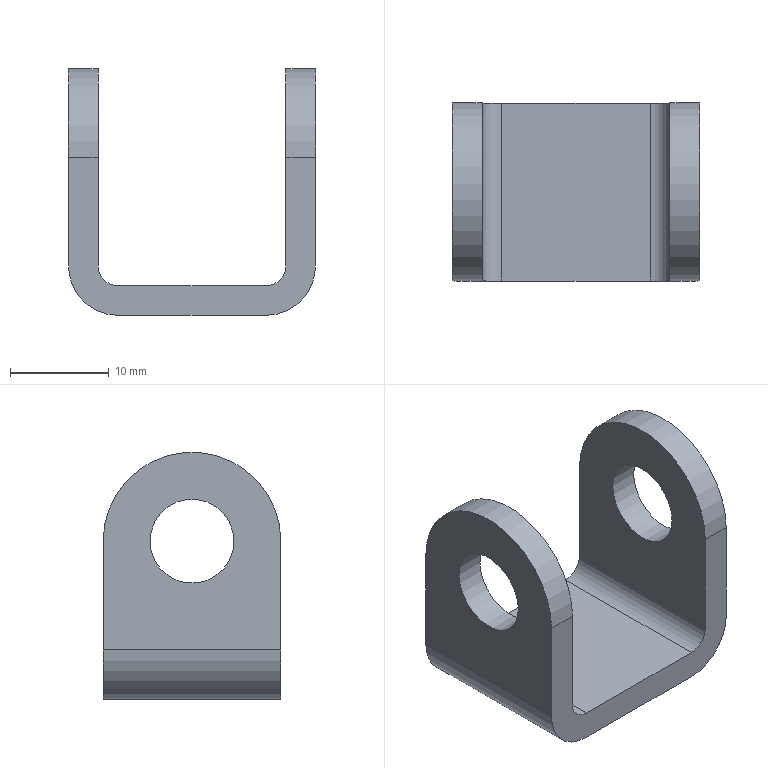Part | NX | features DATUM_CSYS 6, EXTRUDE 5, SKETCH 5, EXTRACT_FACE 4, BLEND 2, Instance Feature 1, Mirror Feature 1 | 1 solid | 16 faces | box 25 x 18 x 25 mm | volume 3015 mm3 | plane 8 | cylinder 8 | commonest cylinder face diameters 4 x2 8.5 x2 10 x2 18 x2
STEP:
#1=CARTESIAN_POINT('',(-12.5,9.,16.));
#2=VERTEX_POINT('',#1);
#3=CARTESIAN_POINT('',(-12.5,9.,5.));
#4=VERTEX_POINT('',#3);
#5=CARTESIAN_POINT('',(-12.5,9.,3.));
#6=DIRECTION('',(0.,0.,-1.));
#7=VECTOR('',#6,1000.);
#8=LINE('',#5,#7);
#9=EDGE_CURVE('',#2,#4,#8,.T.);
#10=ORIENTED_EDGE('',*,*,#9,.T.);
#11=CARTESIAN_POINT('',(-12.5,-9.,5.));
#12=VERTEX_POINT('',#11);
#13=CARTESIAN_POINT('',(-12.5,9.,5.));
#14=DIRECTION('',(0.,-1.,0.));
#15=VECTOR('',#14,1000.);
#16=LINE('',#13,#15);
#17=EDGE_CURVE('',#4,#12,#16,.T.);
#18=ORIENTED_EDGE('',*,*,#17,.T.);
#19=CARTESIAN_POINT('',(-12.5,-9.,16.));
#20=VERTEX_POINT('',#19);
#21=CARTESIAN_POINT('',(-12.5,-9.,3.));
#22=DIRECTION('',(0.,0.,-1.));
#23=VECTOR('',#22,1000.);
#24=LINE('',#21,#23);
#25=EDGE_CURVE('',#20,#12,#24,.T.);
#26=ORIENTED_EDGE('',*,*,#25,.F.);
#27=CARTESIAN_POINT('',(-12.5,0.,16.));
#28=DIRECTION('',(-1.,0.,0.));
#29=DIRECTION('',(0.,-1.,0.));
#30=AXIS2_PLACEMENT_3D('',#27,#28,#29);
#31=CIRCLE('',#30,9.);
#32=EDGE_CURVE('',#20,#2,#31,.T.);
#33=ORIENTED_EDGE('',*,*,#32,.T.);
#34=EDGE_LOOP('',(#10,#18,#26,#33));
#35=FACE_BOUND('',#34,.T.);
#36=CARTESIAN_POINT('',(-12.5,-4.25,16.));
#37=VERTEX_POINT('',#36);
#38=CARTESIAN_POINT('',(-12.5,0.,16.));
#39=DIRECTION('',(-1.,0.,0.));
#40=DIRECTION('',(0.,-1.,0.));
#41=AXIS2_PLACEMENT_3D('',#38,#39,#40);
#42=CIRCLE('',#41,4.25);
#43=EDGE_CURVE('',#37,#37,#42,.T.);
#44=ORIENTED_EDGE('',*,*,#43,.F.);
#45=EDGE_LOOP('',(#44));
#46=FACE_BOUND('',#45,.T.);
#47=CARTESIAN_POINT('',(-12.5,9.,3.));
#48=DIRECTION('',(1.,0.,0.));
#49=DIRECTION('',(0.,1.,0.));
#50=AXIS2_PLACEMENT_3D('',#47,#48,#49);
#51=PLANE('',#50);
#52=ADVANCED_FACE('',(#35,#46),#51,.F.);
#53=CARTESIAN_POINT('',(7.5,9.,3.));
#54=VERTEX_POINT('',#53);
#55=CARTESIAN_POINT('',(-7.5,9.,3.));
#56=VERTEX_POINT('',#55);
#57=CARTESIAN_POINT('',(12.5,9.,3.));
#58=DIRECTION('',(-1.,0.,0.));
#59=VECTOR('',#58,1000.);
#60=LINE('',#57,#59);
#61=EDGE_CURVE('',#54,#56,#60,.T.);
#62=ORIENTED_EDGE('',*,*,#61,.T.);
#63=CARTESIAN_POINT('',(-7.5,-9.,3.));
#64=VERTEX_POINT('',#63);
#65=CARTESIAN_POINT('',(-7.5,0.,3.));
#66=DIRECTION('',(0.,-1.,0.));
#67=VECTOR('',#66,1000.);
#68=LINE('',#65,#67);
#69=EDGE_CURVE('',#56,#64,#68,.T.);
#70=ORIENTED_EDGE('',*,*,#69,.T.);
#71=CARTESIAN_POINT('',(7.5,-9.,3.));
#72=VERTEX_POINT('',#71);
#73=CARTESIAN_POINT('',(-12.5,-9.,3.));
#74=DIRECTION('',(1.,0.,0.));
#75=VECTOR('',#74,1000.);
#76=LINE('',#73,#75);
#77=EDGE_CURVE('',#64,#72,#76,.T.);
#78=ORIENTED_EDGE('',*,*,#77,.T.);
#79=CARTESIAN_POINT('',(7.5,9.,3.));
#80=DIRECTION('',(0.,-1.,0.));
#81=VECTOR('',#80,1000.);
#82=LINE('',#79,#81);
#83=EDGE_CURVE('',#72,#54,#82,.F.);
#84=ORIENTED_EDGE('',*,*,#83,.T.);
#85=EDGE_LOOP('',(#62,#70,#78,#84));
#86=FACE_BOUND('',#85,.T.);
#87=CARTESIAN_POINT('',(0.,0.,3.));
#88=DIRECTION('',(0.,0.,1.));
#89=DIRECTION('',(1.,0.,0.));
#90=AXIS2_PLACEMENT_3D('',#87,#88,#89);
#91=PLANE('',#90);
#92=ADVANCED_FACE('',(#86),#91,.T.);
#93=CARTESIAN_POINT('',(-7.5,-9.,0.));
#94=VERTEX_POINT('',#93);
#95=CARTESIAN_POINT('',(7.5,-9.,0.));
#96=VERTEX_POINT('',#95);
#97=CARTESIAN_POINT('',(-12.5,-9.,0.));
#98=DIRECTION('',(1.,0.,0.));
#99=VECTOR('',#98,1000.);
#100=LINE('',#97,#99);
#101=EDGE_CURVE('',#94,#96,#100,.T.);
#102=ORIENTED_EDGE('',*,*,#101,.T.);
#103=CARTESIAN_POINT('',(12.5,-9.,5.));
#104=VERTEX_POINT('',#103);
#105=CARTESIAN_POINT('',(7.5,-9.,5.));
#106=DIRECTION('',(0.,1.,0.));
#107=DIRECTION('',(-1.,0.,0.));
#108=AXIS2_PLACEMENT_3D('',#105,#106,#107);
#109=CIRCLE('',#108,5.);
#110=EDGE_CURVE('',#96,#104,#109,.F.);
#111=ORIENTED_EDGE('',*,*,#110,.T.);
#112=CARTESIAN_POINT('',(12.5,-9.,16.));
#113=VERTEX_POINT('',#112);
#114=CARTESIAN_POINT('',(12.5,-9.,3.));
#115=DIRECTION('',(0.,0.,-1.));
#116=VECTOR('',#115,1000.);
#117=LINE('',#114,#116);
#118=EDGE_CURVE('',#113,#104,#117,.T.);
#119=ORIENTED_EDGE('',*,*,#118,.F.);
#120=CARTESIAN_POINT('',(9.5,-9.,16.));
#121=VERTEX_POINT('',#120);
#122=CARTESIAN_POINT('',(9.5,-9.,16.));
#123=DIRECTION('',(1.,0.,0.));
#124=VECTOR('',#123,1000.);
#125=LINE('',#122,#124);
#126=EDGE_CURVE('',#121,#113,#125,.T.);
#127=ORIENTED_EDGE('',*,*,#126,.F.);
#128=CARTESIAN_POINT('',(9.5,-9.,5.));
#129=VERTEX_POINT('',#128);
#130=CARTESIAN_POINT('',(9.5,-9.,0.));
#131=DIRECTION('',(0.,0.,1.));
#132=VECTOR('',#131,1000.);
#133=LINE('',#130,#132);
#134=EDGE_CURVE('',#129,#121,#133,.T.);
#135=ORIENTED_EDGE('',*,*,#134,.F.);
#136=CARTESIAN_POINT('',(7.5,-9.,5.));
#137=DIRECTION('',(0.,1.,0.));
#138=DIRECTION('',(-1.,0.,0.));
#139=AXIS2_PLACEMENT_3D('',#136,#137,#138);
#140=CIRCLE('',#139,2.);
#141=EDGE_CURVE('',#129,#72,#140,.T.);
#142=ORIENTED_EDGE('',*,*,#141,.T.);
#143=ORIENTED_EDGE('',*,*,#77,.F.);
#144=CARTESIAN_POINT('',(-9.5,-9.,5.));
#145=VERTEX_POINT('',#144);
#146=CARTESIAN_POINT('',(-7.5,-9.,5.));
#147=DIRECTION('',(0.,1.,0.));
#148=DIRECTION('',(-1.,0.,0.));
#149=AXIS2_PLACEMENT_3D('',#146,#147,#148);
#150=CIRCLE('',#149,2.);
#151=EDGE_CURVE('',#64,#145,#150,.T.);
#152=ORIENTED_EDGE('',*,*,#151,.T.);
#153=CARTESIAN_POINT('',(-9.5,-9.,16.));
#154=VERTEX_POINT('',#153);
#155=CARTESIAN_POINT('',(-9.5,-9.,0.));
#156=DIRECTION('',(0.,0.,1.));
#157=VECTOR('',#156,1000.);
#158=LINE('',#155,#157);
#159=EDGE_CURVE('',#145,#154,#158,.T.);
#160=ORIENTED_EDGE('',*,*,#159,.T.);
#161=CARTESIAN_POINT('',(-9.5,-9.,16.));
#162=DIRECTION('',(-1.,0.,0.));
#163=VECTOR('',#162,1000.);
#164=LINE('',#161,#163);
#165=EDGE_CURVE('',#154,#20,#164,.T.);
#166=ORIENTED_EDGE('',*,*,#165,.T.);
#167=ORIENTED_EDGE('',*,*,#25,.T.);
#168=CARTESIAN_POINT('',(-7.5,-9.,5.));
#169=DIRECTION('',(0.,1.,0.));
#170=DIRECTION('',(-1.,0.,0.));
#171=AXIS2_PLACEMENT_3D('',#168,#169,#170);
#172=CIRCLE('',#171,5.);
#173=EDGE_CURVE('',#12,#94,#172,.F.);
#174=ORIENTED_EDGE('',*,*,#173,.T.);
#175=EDGE_LOOP('',(#102,#111,#119,#127,#135,#142,#143,#152,#160,#166,#167,#174));
#176=FACE_BOUND('',#175,.T.);
#177=CARTESIAN_POINT('',(-12.5,-9.,3.));
#178=DIRECTION('',(0.,1.,0.));
#179=DIRECTION('',(-1.,0.,0.));
#180=AXIS2_PLACEMENT_3D('',#177,#178,#179);
#181=PLANE('',#180);
#182=ADVANCED_FACE('',(#176),#181,.F.);
#183=CARTESIAN_POINT('',(12.5,-4.25,16.));
#184=VERTEX_POINT('',#183);
#185=CARTESIAN_POINT('',(12.5,0.,16.));
#186=DIRECTION('',(-1.,0.,0.));
#187=DIRECTION('',(0.,-1.,0.));
#188=AXIS2_PLACEMENT_3D('',#185,#186,#187);
#189=CIRCLE('',#188,4.25);
#190=EDGE_CURVE('',#184,#184,#189,.T.);
#191=ORIENTED_EDGE('',*,*,#190,.T.);
#192=EDGE_LOOP('',(#191));
#193=FACE_BOUND('',#192,.T.);
#194=ORIENTED_EDGE('',*,*,#118,.T.);
#195=CARTESIAN_POINT('',(12.5,9.,5.));
#196=VERTEX_POINT('',#195);
#197=CARTESIAN_POINT('',(12.5,-9.,5.));
#198=DIRECTION('',(0.,1.,0.));
#199=VECTOR('',#198,1000.);
#200=LINE('',#197,#199);
#201=EDGE_CURVE('',#104,#196,#200,.T.);
#202=ORIENTED_EDGE('',*,*,#201,.T.);
#203=CARTESIAN_POINT('',(12.5,9.,16.));
#204=VERTEX_POINT('',#203);
#205=CARTESIAN_POINT('',(12.5,9.,3.));
#206=DIRECTION('',(0.,0.,-1.));
#207=VECTOR('',#206,1000.);
#208=LINE('',#205,#207);
#209=EDGE_CURVE('',#204,#196,#208,.T.);
#210=ORIENTED_EDGE('',*,*,#209,.F.);
#211=CARTESIAN_POINT('',(12.5,0.,16.));
#212=DIRECTION('',(-1.,0.,0.));
#213=DIRECTION('',(0.,-1.,0.));
#214=AXIS2_PLACEMENT_3D('',#211,#212,#213);
#215=CIRCLE('',#214,9.);
#216=EDGE_CURVE('',#113,#204,#215,.T.);
#217=ORIENTED_EDGE('',*,*,#216,.F.);
#218=EDGE_LOOP('',(#194,#202,#210,#217));
#219=FACE_BOUND('',#218,.T.);
#220=CARTESIAN_POINT('',(12.5,-9.,3.));
#221=DIRECTION('',(-1.,0.,0.));
#222=DIRECTION('',(0.,-1.,0.));
#223=AXIS2_PLACEMENT_3D('',#220,#221,#222);
#224=PLANE('',#223);
#225=ADVANCED_FACE('',(#193,#219),#224,.F.);
#226=ORIENTED_EDGE('',*,*,#209,.T.);
#227=CARTESIAN_POINT('',(7.5,9.,0.));
#228=VERTEX_POINT('',#227);
#229=CARTESIAN_POINT('',(7.5,9.,5.));
#230=DIRECTION('',(0.,-1.,0.));
#231=DIRECTION('',(0.,0.,-1.));
#232=AXIS2_PLACEMENT_3D('',#229,#230,#231);
#233=CIRCLE('',#232,5.);
#234=EDGE_CURVE('',#196,#228,#233,.F.);
#235=ORIENTED_EDGE('',*,*,#234,.T.);
#236=CARTESIAN_POINT('',(-7.5,9.,0.));
#237=VERTEX_POINT('',#236);
#238=CARTESIAN_POINT('',(12.5,9.,0.));
#239=DIRECTION('',(-1.,0.,0.));
#240=VECTOR('',#239,1000.);
#241=LINE('',#238,#240);
#242=EDGE_CURVE('',#228,#237,#241,.T.);
#243=ORIENTED_EDGE('',*,*,#242,.T.);
#244=CARTESIAN_POINT('',(-7.5,9.,5.));
#245=DIRECTION('',(0.,-1.,0.));
#246=DIRECTION('',(0.,0.,-1.));
#247=AXIS2_PLACEMENT_3D('',#244,#245,#246);
#248=CIRCLE('',#247,5.);
#249=EDGE_CURVE('',#237,#4,#248,.F.);
#250=ORIENTED_EDGE('',*,*,#249,.T.);
#251=ORIENTED_EDGE('',*,*,#9,.F.);
#252=CARTESIAN_POINT('',(-9.5,9.,16.));
#253=VERTEX_POINT('',#252);
#254=CARTESIAN_POINT('',(-9.5,9.,16.));
#255=DIRECTION('',(-1.,0.,0.));
#256=VECTOR('',#255,1000.);
#257=LINE('',#254,#256);
#258=EDGE_CURVE('',#253,#2,#257,.T.);
#259=ORIENTED_EDGE('',*,*,#258,.F.);
#260=CARTESIAN_POINT('',(-9.5,9.,5.));
#261=VERTEX_POINT('',#260);
#262=CARTESIAN_POINT('',(-9.5,9.,16.));
#263=DIRECTION('',(0.,0.,-1.));
#264=VECTOR('',#263,1000.);
#265=LINE('',#262,#264);
#266=EDGE_CURVE('',#253,#261,#265,.T.);
#267=ORIENTED_EDGE('',*,*,#266,.T.);
#268=CARTESIAN_POINT('',(-7.5,9.,5.));
#269=DIRECTION('',(0.,-1.,0.));
#270=DIRECTION('',(0.,0.,-1.));
#271=AXIS2_PLACEMENT_3D('',#268,#269,#270);
#272=CIRCLE('',#271,2.);
#273=EDGE_CURVE('',#261,#56,#272,.T.);
#274=ORIENTED_EDGE('',*,*,#273,.T.);
#275=ORIENTED_EDGE('',*,*,#61,.F.);
#276=CARTESIAN_POINT('',(9.5,9.,5.));
#277=VERTEX_POINT('',#276);
#278=CARTESIAN_POINT('',(7.5,9.,5.));
#279=DIRECTION('',(0.,-1.,0.));
#280=DIRECTION('',(0.,0.,-1.));
#281=AXIS2_PLACEMENT_3D('',#278,#279,#280);
#282=CIRCLE('',#281,2.);
#283=EDGE_CURVE('',#54,#277,#282,.T.);
#284=ORIENTED_EDGE('',*,*,#283,.T.);
#285=CARTESIAN_POINT('',(9.5,9.,16.));
#286=VERTEX_POINT('',#285);
#287=CARTESIAN_POINT('',(9.5,9.,16.));
#288=DIRECTION('',(0.,0.,-1.));
#289=VECTOR('',#288,1000.);
#290=LINE('',#287,#289);
#291=EDGE_CURVE('',#286,#277,#290,.T.);
#292=ORIENTED_EDGE('',*,*,#291,.F.);
#293=CARTESIAN_POINT('',(9.5,9.,16.));
#294=DIRECTION('',(1.,0.,0.));
#295=VECTOR('',#294,1000.);
#296=LINE('',#293,#295);
#297=EDGE_CURVE('',#286,#204,#296,.T.);
#298=ORIENTED_EDGE('',*,*,#297,.T.);
#299=EDGE_LOOP('',(#226,#235,#243,#250,#251,#259,#267,#274,#275,#284,#292,#298));
#300=FACE_BOUND('',#299,.T.);
#301=CARTESIAN_POINT('',(12.5,9.,3.));
#302=DIRECTION('',(0.,-1.,0.));
#303=DIRECTION('',(0.,0.,-1.));
#304=AXIS2_PLACEMENT_3D('',#301,#302,#303);
#305=PLANE('',#304);
#306=ADVANCED_FACE('',(#300),#305,.F.);
#307=ORIENTED_EDGE('',*,*,#242,.F.);
#308=CARTESIAN_POINT('',(7.5,0.,0.));
#309=DIRECTION('',(0.,1.,0.));
#310=VECTOR('',#309,1000.);
#311=LINE('',#308,#310);
#312=EDGE_CURVE('',#228,#96,#311,.F.);
#313=ORIENTED_EDGE('',*,*,#312,.T.);
#314=ORIENTED_EDGE('',*,*,#101,.F.);
#315=CARTESIAN_POINT('',(-7.5,0.,0.));
#316=DIRECTION('',(0.,-1.,0.));
#317=VECTOR('',#316,1000.);
#318=LINE('',#315,#317);
#319=EDGE_CURVE('',#94,#237,#318,.F.);
#320=ORIENTED_EDGE('',*,*,#319,.T.);
#321=EDGE_LOOP('',(#307,#313,#314,#320));
#322=FACE_BOUND('',#321,.T.);
#323=CARTESIAN_POINT('',(0.,0.,0.));
#324=DIRECTION('',(0.,0.,1.));
#325=DIRECTION('',(1.,0.,0.));
#326=AXIS2_PLACEMENT_3D('',#323,#324,#325);
#327=PLANE('',#326);
#328=ADVANCED_FACE('',(#322),#327,.F.);
#329=ORIENTED_EDGE('',*,*,#32,.F.);
#330=ORIENTED_EDGE('',*,*,#165,.F.);
#331=CARTESIAN_POINT('',(-9.5,0.,16.));
#332=DIRECTION('',(-1.,0.,0.));
#333=DIRECTION('',(0.,-1.,0.));
#334=AXIS2_PLACEMENT_3D('',#331,#332,#333);
#335=CIRCLE('',#334,9.);
#336=EDGE_CURVE('',#154,#253,#335,.T.);
#337=ORIENTED_EDGE('',*,*,#336,.T.);
#338=ORIENTED_EDGE('',*,*,#258,.T.);
#339=EDGE_LOOP('',(#329,#330,#337,#338));
#340=FACE_BOUND('',#339,.T.);
#341=CARTESIAN_POINT('',(-9.5,0.,16.));
#342=DIRECTION('',(-1.,0.,0.));
#343=DIRECTION('',(0.,0.,1.));
#344=AXIS2_PLACEMENT_3D('',#341,#342,#343);
#345=CYLINDRICAL_SURFACE('',#344,9.);
#346=ADVANCED_FACE('',(#340),#345,.T.);
#347=CARTESIAN_POINT('',(-9.5,-4.25,16.));
#348=VERTEX_POINT('',#347);
#349=CARTESIAN_POINT('',(-9.5,0.,16.));
#350=DIRECTION('',(-1.,0.,0.));
#351=DIRECTION('',(0.,-1.,0.));
#352=AXIS2_PLACEMENT_3D('',#349,#350,#351);
#353=CIRCLE('',#352,4.25);
#354=EDGE_CURVE('',#348,#348,#353,.T.);
#355=ORIENTED_EDGE('',*,*,#354,.T.);
#356=EDGE_LOOP('',(#355));
#357=FACE_BOUND('',#356,.T.);
#358=ORIENTED_EDGE('',*,*,#159,.F.);
#359=CARTESIAN_POINT('',(-9.5,0.,5.));
#360=DIRECTION('',(0.,-1.,0.));
#361=VECTOR('',#360,1000.);
#362=LINE('',#359,#361);
#363=EDGE_CURVE('',#145,#261,#362,.F.);
#364=ORIENTED_EDGE('',*,*,#363,.T.);
#365=ORIENTED_EDGE('',*,*,#266,.F.);
#366=ORIENTED_EDGE('',*,*,#336,.F.);
#367=EDGE_LOOP('',(#358,#364,#365,#366));
#368=FACE_BOUND('',#367,.T.);
#369=CARTESIAN_POINT('',(-9.5,0.,16.));
#370=DIRECTION('',(-1.,0.,0.));
#371=DIRECTION('',(0.,0.,1.));
#372=AXIS2_PLACEMENT_3D('',#369,#370,#371);
#373=PLANE('',#372);
#374=ADVANCED_FACE('',(#357,#368),#373,.F.);
#375=ORIENTED_EDGE('',*,*,#354,.F.);
#376=EDGE_LOOP('',(#375));
#377=FACE_BOUND('',#376,.T.);
#378=ORIENTED_EDGE('',*,*,#43,.T.);
#379=EDGE_LOOP('',(#378));
#380=FACE_BOUND('',#379,.T.);
#381=CARTESIAN_POINT('',(-9.5,0.,16.));
#382=DIRECTION('',(-1.,0.,0.));
#383=DIRECTION('',(0.,0.,1.));
#384=AXIS2_PLACEMENT_3D('',#381,#382,#383);
#385=CYLINDRICAL_SURFACE('',#384,4.25);
#386=ADVANCED_FACE('',(#377,#380),#385,.F.);
#387=ORIENTED_EDGE('',*,*,#216,.T.);
#388=ORIENTED_EDGE('',*,*,#297,.F.);
#389=CARTESIAN_POINT('',(9.5,0.,16.));
#390=DIRECTION('',(-1.,0.,0.));
#391=DIRECTION('',(0.,-1.,0.));
#392=AXIS2_PLACEMENT_3D('',#389,#390,#391);
#393=CIRCLE('',#392,9.);
#394=EDGE_CURVE('',#286,#121,#393,.F.);
#395=ORIENTED_EDGE('',*,*,#394,.T.);
#396=ORIENTED_EDGE('',*,*,#126,.T.);
#397=EDGE_LOOP('',(#387,#388,#395,#396));
#398=FACE_BOUND('',#397,.T.);
#399=CARTESIAN_POINT('',(9.5,0.,16.));
#400=DIRECTION('',(1.,0.,0.));
#401=DIRECTION('',(0.,0.,-1.));
#402=AXIS2_PLACEMENT_3D('',#399,#400,#401);
#403=CYLINDRICAL_SURFACE('',#402,9.);
#404=ADVANCED_FACE('',(#398),#403,.T.);
#405=CARTESIAN_POINT('',(9.5,-4.25,16.));
#406=VERTEX_POINT('',#405);
#407=CARTESIAN_POINT('',(9.5,0.,16.));
#408=DIRECTION('',(-1.,0.,0.));
#409=DIRECTION('',(0.,-1.,0.));
#410=AXIS2_PLACEMENT_3D('',#407,#408,#409);
#411=CIRCLE('',#410,4.25);
#412=EDGE_CURVE('',#406,#406,#411,.F.);
#413=ORIENTED_EDGE('',*,*,#412,.T.);
#414=EDGE_LOOP('',(#413));
#415=FACE_BOUND('',#414,.T.);
#416=ORIENTED_EDGE('',*,*,#291,.T.);
#417=CARTESIAN_POINT('',(9.5,-9.,5.));
#418=DIRECTION('',(0.,-1.,0.));
#419=VECTOR('',#418,1000.);
#420=LINE('',#417,#419);
#421=EDGE_CURVE('',#277,#129,#420,.T.);
#422=ORIENTED_EDGE('',*,*,#421,.T.);
#423=ORIENTED_EDGE('',*,*,#134,.T.);
#424=ORIENTED_EDGE('',*,*,#394,.F.);
#425=EDGE_LOOP('',(#416,#422,#423,#424));
#426=FACE_BOUND('',#425,.T.);
#427=CARTESIAN_POINT('',(9.5,0.,16.));
#428=DIRECTION('',(-1.,0.,0.));
#429=DIRECTION('',(0.,0.,1.));
#430=AXIS2_PLACEMENT_3D('',#427,#428,#429);
#431=PLANE('',#430);
#432=ADVANCED_FACE('',(#415,#426),#431,.T.);
#433=ORIENTED_EDGE('',*,*,#412,.F.);
#434=EDGE_LOOP('',(#433));
#435=FACE_BOUND('',#434,.T.);
#436=ORIENTED_EDGE('',*,*,#190,.F.);
#437=EDGE_LOOP('',(#436));
#438=FACE_BOUND('',#437,.T.);
#439=CARTESIAN_POINT('',(9.5,0.,16.));
#440=DIRECTION('',(1.,0.,0.));
#441=DIRECTION('',(0.,0.,-1.));
#442=AXIS2_PLACEMENT_3D('',#439,#440,#441);
#443=CYLINDRICAL_SURFACE('',#442,4.25);
#444=ADVANCED_FACE('',(#435,#438),#443,.F.);
#445=ORIENTED_EDGE('',*,*,#273,.F.);
#446=ORIENTED_EDGE('',*,*,#363,.F.);
#447=ORIENTED_EDGE('',*,*,#151,.F.);
#448=ORIENTED_EDGE('',*,*,#69,.F.);
#449=EDGE_LOOP('',(#445,#446,#447,#448));
#450=FACE_BOUND('',#449,.T.);
#451=CARTESIAN_POINT('',(-7.5,0.,5.));
#452=DIRECTION('',(0.,-1.,0.));
#453=DIRECTION('',(0.,0.,-1.));
#454=AXIS2_PLACEMENT_3D('',#451,#452,#453);
#455=CYLINDRICAL_SURFACE('',#454,2.);
#456=ADVANCED_FACE('',(#450),#455,.F.);
#457=ORIENTED_EDGE('',*,*,#283,.F.);
#458=ORIENTED_EDGE('',*,*,#83,.F.);
#459=ORIENTED_EDGE('',*,*,#141,.F.);
#460=ORIENTED_EDGE('',*,*,#421,.F.);
#461=EDGE_LOOP('',(#457,#458,#459,#460));
#462=FACE_BOUND('',#461,.T.);
#463=CARTESIAN_POINT('',(7.5,0.,5.));
#464=DIRECTION('',(0.,1.,0.));
#465=DIRECTION('',(0.,0.,1.));
#466=AXIS2_PLACEMENT_3D('',#463,#464,#465);
#467=CYLINDRICAL_SURFACE('',#466,2.);
#468=ADVANCED_FACE('',(#462),#467,.F.);
#469=ORIENTED_EDGE('',*,*,#110,.F.);
#470=ORIENTED_EDGE('',*,*,#312,.F.);
#471=ORIENTED_EDGE('',*,*,#234,.F.);
#472=ORIENTED_EDGE('',*,*,#201,.F.);
#473=EDGE_LOOP('',(#469,#470,#471,#472));
#474=FACE_BOUND('',#473,.T.);
#475=CARTESIAN_POINT('',(7.5,-9.,5.));
#476=DIRECTION('',(0.,1.,0.));
#477=DIRECTION('',(-1.,0.,0.));
#478=AXIS2_PLACEMENT_3D('',#475,#476,#477);
#479=CYLINDRICAL_SURFACE('',#478,5.);
#480=ADVANCED_FACE('',(#474),#479,.T.);
#481=ORIENTED_EDGE('',*,*,#249,.F.);
#482=ORIENTED_EDGE('',*,*,#319,.F.);
#483=ORIENTED_EDGE('',*,*,#173,.F.);
#484=ORIENTED_EDGE('',*,*,#17,.F.);
#485=EDGE_LOOP('',(#481,#482,#483,#484));
#486=FACE_BOUND('',#485,.T.);
#487=CARTESIAN_POINT('',(-7.5,9.,5.));
#488=DIRECTION('',(0.,-1.,0.));
#489=DIRECTION('',(1.,0.,0.));
#490=AXIS2_PLACEMENT_3D('',#487,#488,#489);
#491=CYLINDRICAL_SURFACE('',#490,5.);
#492=ADVANCED_FACE('',(#486),#491,.T.);
#493=CLOSED_SHELL('',(#52,#92,#182,#225,#306,#328,#346,#374,#386,#404,#432,#444,#456,#468,#480,#492));
#494=MANIFOLD_SOLID_BREP('',#493);
#495=(LENGTH_UNIT()NAMED_UNIT(*)SI_UNIT(.MILLI.,.METRE.));
#496=UNCERTAINTY_MEASURE_WITH_UNIT(LENGTH_MEASURE(0.00001),#495,'','');
#497=(NAMED_UNIT(*)PLANE_ANGLE_UNIT()SI_UNIT($,.RADIAN.));
#498=(NAMED_UNIT(*)SI_UNIT($,.STERADIAN.)SOLID_ANGLE_UNIT());
#499=(GEOMETRIC_REPRESENTATION_CONTEXT(3)GLOBAL_UNCERTAINTY_ASSIGNED_CONTEXT((#496))GLOBAL_UNIT_ASSIGNED_CONTEXT((#495,#497,#498))REPRESENTATION_CONTEXT('',''));
#500=ADVANCED_BREP_SHAPE_REPRESENTATION('',(#494),#499);